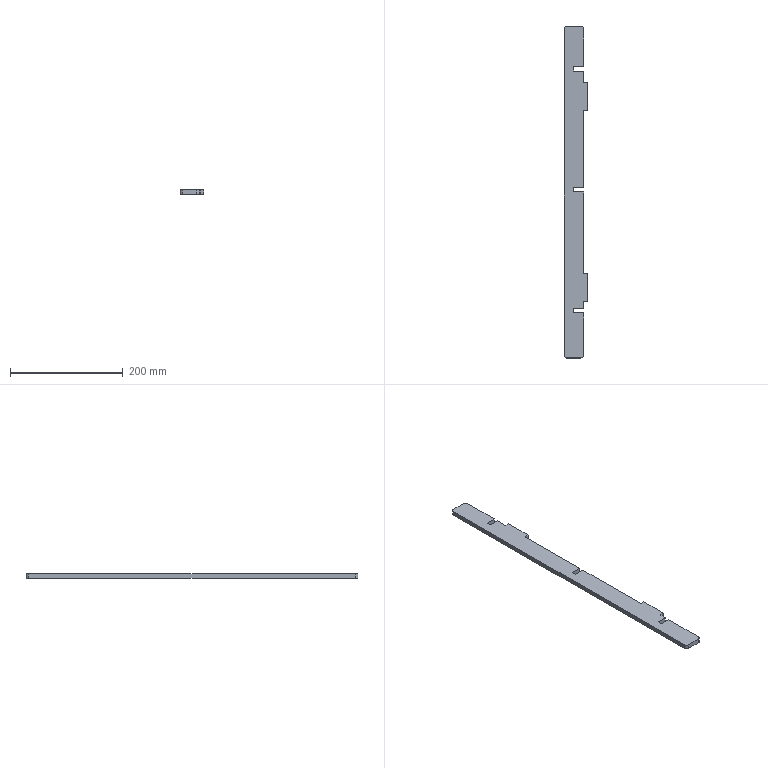Part | SolidWorks | features Fillet 2, FlatPattern 1, ICE 1, SMBaseFlange 1, SheetMetal 1 | 1 solid | 42 faces | box 42.5 x 590 x 8 mm | volume 167562 mm3 | plane 26 | cylinder 16 | commonest cylinder face diameters 2 x8 1 x4 10 x4
STEP:
#1=CARTESIAN_POINT('',(-612.5,244.764,0.));
#2=VERTEX_POINT('',#1);
#3=CARTESIAN_POINT('',(-612.5,263.685,0.));
#4=VERTEX_POINT('',#3);
#5=CARTESIAN_POINT('',(-612.5,243.685,0.));
#6=DIRECTION('',(0.,1.,0.));
#7=VECTOR('',#6,1000.);
#8=LINE('',#5,#7);
#9=EDGE_CURVE('',#2,#4,#8,.T.);
#10=ORIENTED_EDGE('',*,*,#9,.F.);
#11=CARTESIAN_POINT('',(-612.5,244.764,-8.));
#12=VERTEX_POINT('',#11);
#13=CARTESIAN_POINT('',(-612.5,244.764,-8.));
#14=DIRECTION('',(0.,0.,-1.));
#15=VECTOR('',#14,1000.);
#16=LINE('',#13,#15);
#17=EDGE_CURVE('',#2,#12,#16,.T.);
#18=ORIENTED_EDGE('',*,*,#17,.T.);
#19=CARTESIAN_POINT('',(-612.5,263.685,-8.));
#20=VERTEX_POINT('',#19);
#21=CARTESIAN_POINT('',(-612.5,243.685,-8.));
#22=DIRECTION('',(0.,1.,0.));
#23=VECTOR('',#22,1000.);
#24=LINE('',#21,#23);
#25=EDGE_CURVE('',#12,#20,#24,.T.);
#26=ORIENTED_EDGE('',*,*,#25,.T.);
#27=CARTESIAN_POINT('',(-612.5,263.685,-8.));
#28=DIRECTION('',(0.,0.,1.));
#29=VECTOR('',#28,1000.);
#30=LINE('',#27,#29);
#31=EDGE_CURVE('',#20,#4,#30,.T.);
#32=ORIENTED_EDGE('',*,*,#31,.T.);
#33=EDGE_LOOP('',(#10,#18,#26,#32));
#34=FACE_OUTER_BOUND('',#33,.T.);
#35=CARTESIAN_POINT('',(-612.5,243.685,-8.));
#36=DIRECTION('',(1.,0.,0.));
#37=DIRECTION('',(0.,1.,0.));
#38=AXIS2_PLACEMENT_3D('',#35,#36,#37);
#39=PLANE('',#38);
#40=ADVANCED_FACE('',(#34),#39,.T.);
#41=CARTESIAN_POINT('',(-605.,243.685,-8.));
#42=VERTEX_POINT('',#41);
#43=CARTESIAN_POINT('',(-611.421,243.685,-8.));
#44=VERTEX_POINT('',#43);
#45=CARTESIAN_POINT('',(-612.5,243.685,-8.));
#46=DIRECTION('',(-1.,0.,0.));
#47=VECTOR('',#46,1000.);
#48=LINE('',#45,#47);
#49=EDGE_CURVE('',#42,#44,#48,.T.);
#50=ORIENTED_EDGE('',*,*,#49,.T.);
#51=CARTESIAN_POINT('',(-611.421,243.685,0.));
#52=VERTEX_POINT('',#51);
#53=CARTESIAN_POINT('',(-611.421,243.685,-8.));
#54=DIRECTION('',(0.,0.,1.));
#55=VECTOR('',#54,1000.);
#56=LINE('',#53,#55);
#57=EDGE_CURVE('',#44,#52,#56,.T.);
#58=ORIENTED_EDGE('',*,*,#57,.T.);
#59=CARTESIAN_POINT('',(-605.,243.685,0.));
#60=VERTEX_POINT('',#59);
#61=CARTESIAN_POINT('',(-612.5,243.685,0.));
#62=DIRECTION('',(-1.,0.,0.));
#63=VECTOR('',#62,1000.);
#64=LINE('',#61,#63);
#65=EDGE_CURVE('',#60,#52,#64,.T.);
#66=ORIENTED_EDGE('',*,*,#65,.F.);
#67=CARTESIAN_POINT('',(-605.,243.685,-8.));
#68=DIRECTION('',(0.,0.,1.));
#69=VECTOR('',#68,1000.);
#70=LINE('',#67,#69);
#71=EDGE_CURVE('',#42,#60,#70,.T.);
#72=ORIENTED_EDGE('',*,*,#71,.F.);
#73=EDGE_LOOP('',(#50,#58,#66,#72));
#74=FACE_OUTER_BOUND('',#73,.T.);
#75=CARTESIAN_POINT('',(-612.5,243.685,-8.));
#76=DIRECTION('',(0.,1.,0.));
#77=DIRECTION('',(0.,0.,1.));
#78=AXIS2_PLACEMENT_3D('',#75,#76,#77);
#79=PLANE('',#78);
#80=ADVANCED_FACE('',(#74),#79,.T.);
#81=CARTESIAN_POINT('',(-611.421,193.685,0.));
#82=VERTEX_POINT('',#81);
#83=CARTESIAN_POINT('',(-605.,193.685,0.));
#84=VERTEX_POINT('',#83);
#85=CARTESIAN_POINT('',(-605.,193.685,0.));
#86=DIRECTION('',(1.,0.,0.));
#87=VECTOR('',#86,1000.);
#88=LINE('',#85,#87);
#89=EDGE_CURVE('',#82,#84,#88,.T.);
#90=ORIENTED_EDGE('',*,*,#89,.F.);
#91=CARTESIAN_POINT('',(-611.421,193.685,-8.));
#92=VERTEX_POINT('',#91);
#93=CARTESIAN_POINT('',(-611.421,193.685,-8.));
#94=DIRECTION('',(0.,0.,-1.));
#95=VECTOR('',#94,1000.);
#96=LINE('',#93,#95);
#97=EDGE_CURVE('',#82,#92,#96,.T.);
#98=ORIENTED_EDGE('',*,*,#97,.T.);
#99=CARTESIAN_POINT('',(-605.,193.685,-8.));
#100=VERTEX_POINT('',#99);
#101=CARTESIAN_POINT('',(-605.,193.685,-8.));
#102=DIRECTION('',(1.,0.,0.));
#103=VECTOR('',#102,1000.);
#104=LINE('',#101,#103);
#105=EDGE_CURVE('',#92,#100,#104,.T.);
#106=ORIENTED_EDGE('',*,*,#105,.T.);
#107=CARTESIAN_POINT('',(-605.,193.685,-8.));
#108=DIRECTION('',(0.,0.,1.));
#109=VECTOR('',#108,1000.);
#110=LINE('',#107,#109);
#111=EDGE_CURVE('',#100,#84,#110,.T.);
#112=ORIENTED_EDGE('',*,*,#111,.T.);
#113=EDGE_LOOP('',(#90,#98,#106,#112));
#114=FACE_OUTER_BOUND('',#113,.T.);
#115=CARTESIAN_POINT('',(-605.,193.685,-8.));
#116=DIRECTION('',(0.,-1.,0.));
#117=DIRECTION('',(0.,0.,-1.));
#118=AXIS2_PLACEMENT_3D('',#115,#116,#117);
#119=PLANE('',#118);
#120=ADVANCED_FACE('',(#114),#119,.T.);
#121=CARTESIAN_POINT('',(-612.5,56.685,-8.));
#122=VERTEX_POINT('',#121);
#123=CARTESIAN_POINT('',(-612.5,192.605,-8.));
#124=VERTEX_POINT('',#123);
#125=CARTESIAN_POINT('',(-612.5,56.685,-8.));
#126=DIRECTION('',(0.,1.,0.));
#127=VECTOR('',#126,1000.);
#128=LINE('',#125,#127);
#129=EDGE_CURVE('',#122,#124,#128,.T.);
#130=ORIENTED_EDGE('',*,*,#129,.T.);
#131=CARTESIAN_POINT('',(-612.5,192.605,0.));
#132=VERTEX_POINT('',#131);
#133=CARTESIAN_POINT('',(-612.5,192.605,-8.));
#134=DIRECTION('',(0.,0.,1.));
#135=VECTOR('',#134,1000.);
#136=LINE('',#133,#135);
#137=EDGE_CURVE('',#124,#132,#136,.T.);
#138=ORIENTED_EDGE('',*,*,#137,.T.);
#139=CARTESIAN_POINT('',(-612.5,56.685,0.));
#140=VERTEX_POINT('',#139);
#141=CARTESIAN_POINT('',(-612.5,56.685,0.));
#142=DIRECTION('',(0.,1.,0.));
#143=VECTOR('',#142,1000.);
#144=LINE('',#141,#143);
#145=EDGE_CURVE('',#140,#132,#144,.T.);
#146=ORIENTED_EDGE('',*,*,#145,.F.);
#147=CARTESIAN_POINT('',(-612.5,56.685,-8.));
#148=DIRECTION('',(0.,0.,1.));
#149=VECTOR('',#148,1000.);
#150=LINE('',#147,#149);
#151=EDGE_CURVE('',#122,#140,#150,.T.);
#152=ORIENTED_EDGE('',*,*,#151,.F.);
#153=EDGE_LOOP('',(#130,#138,#146,#152));
#154=FACE_OUTER_BOUND('',#153,.T.);
#155=CARTESIAN_POINT('',(-612.5,56.685,-8.));
#156=DIRECTION('',(1.,0.,0.));
#157=DIRECTION('',(0.,1.,0.));
#158=AXIS2_PLACEMENT_3D('',#155,#156,#157);
#159=PLANE('',#158);
#160=ADVANCED_FACE('',(#154),#159,.T.);
#161=CARTESIAN_POINT('',(-612.5,-95.236,0.));
#162=VERTEX_POINT('',#161);
#163=CARTESIAN_POINT('',(-612.5,48.685,0.));
#164=VERTEX_POINT('',#163);
#165=CARTESIAN_POINT('',(-612.5,-96.315,0.));
#166=DIRECTION('',(0.,1.,0.));
#167=VECTOR('',#166,1000.);
#168=LINE('',#165,#167);
#169=EDGE_CURVE('',#162,#164,#168,.T.);
#170=ORIENTED_EDGE('',*,*,#169,.F.);
#171=CARTESIAN_POINT('',(-612.5,-95.236,-8.));
#172=VERTEX_POINT('',#171);
#173=CARTESIAN_POINT('',(-612.5,-95.236,-8.));
#174=DIRECTION('',(0.,0.,-1.));
#175=VECTOR('',#174,1000.);
#176=LINE('',#173,#175);
#177=EDGE_CURVE('',#162,#172,#176,.T.);
#178=ORIENTED_EDGE('',*,*,#177,.T.);
#179=CARTESIAN_POINT('',(-612.5,48.685,-8.));
#180=VERTEX_POINT('',#179);
#181=CARTESIAN_POINT('',(-612.5,-96.315,-8.));
#182=DIRECTION('',(0.,1.,0.));
#183=VECTOR('',#182,1000.);
#184=LINE('',#181,#183);
#185=EDGE_CURVE('',#172,#180,#184,.T.);
#186=ORIENTED_EDGE('',*,*,#185,.T.);
#187=CARTESIAN_POINT('',(-612.5,48.685,-8.));
#188=DIRECTION('',(0.,0.,1.));
#189=VECTOR('',#188,1000.);
#190=LINE('',#187,#189);
#191=EDGE_CURVE('',#180,#164,#190,.T.);
#192=ORIENTED_EDGE('',*,*,#191,.T.);
#193=EDGE_LOOP('',(#170,#178,#186,#192));
#194=FACE_OUTER_BOUND('',#193,.T.);
#195=CARTESIAN_POINT('',(-612.5,-96.315,-8.));
#196=DIRECTION('',(1.,0.,0.));
#197=DIRECTION('',(0.,1.,0.));
#198=AXIS2_PLACEMENT_3D('',#195,#196,#197);
#199=PLANE('',#198);
#200=ADVANCED_FACE('',(#194),#199,.T.);
#201=CARTESIAN_POINT('',(-605.,-96.315,-8.));
#202=VERTEX_POINT('',#201);
#203=CARTESIAN_POINT('',(-611.421,-96.315,-8.));
#204=VERTEX_POINT('',#203);
#205=CARTESIAN_POINT('',(-612.5,-96.315,-8.));
#206=DIRECTION('',(-1.,0.,0.));
#207=VECTOR('',#206,1000.);
#208=LINE('',#205,#207);
#209=EDGE_CURVE('',#202,#204,#208,.T.);
#210=ORIENTED_EDGE('',*,*,#209,.T.);
#211=CARTESIAN_POINT('',(-611.421,-96.315,0.));
#212=VERTEX_POINT('',#211);
#213=CARTESIAN_POINT('',(-611.421,-96.315,-8.));
#214=DIRECTION('',(0.,0.,1.));
#215=VECTOR('',#214,1000.);
#216=LINE('',#213,#215);
#217=EDGE_CURVE('',#204,#212,#216,.T.);
#218=ORIENTED_EDGE('',*,*,#217,.T.);
#219=CARTESIAN_POINT('',(-605.,-96.315,0.));
#220=VERTEX_POINT('',#219);
#221=CARTESIAN_POINT('',(-612.5,-96.315,0.));
#222=DIRECTION('',(-1.,0.,0.));
#223=VECTOR('',#222,1000.);
#224=LINE('',#221,#223);
#225=EDGE_CURVE('',#220,#212,#224,.T.);
#226=ORIENTED_EDGE('',*,*,#225,.F.);
#227=CARTESIAN_POINT('',(-605.,-96.315,-8.));
#228=DIRECTION('',(0.,0.,1.));
#229=VECTOR('',#228,1000.);
#230=LINE('',#227,#229);
#231=EDGE_CURVE('',#202,#220,#230,.T.);
#232=ORIENTED_EDGE('',*,*,#231,.F.);
#233=EDGE_LOOP('',(#210,#218,#226,#232));
#234=FACE_OUTER_BOUND('',#233,.T.);
#235=CARTESIAN_POINT('',(-612.5,-96.315,-8.));
#236=DIRECTION('',(0.,1.,0.));
#237=DIRECTION('',(0.,0.,1.));
#238=AXIS2_PLACEMENT_3D('',#235,#236,#237);
#239=PLANE('',#238);
#240=ADVANCED_FACE('',(#234),#239,.T.);
#241=CARTESIAN_POINT('',(-611.421,-146.315,0.));
#242=VERTEX_POINT('',#241);
#243=CARTESIAN_POINT('',(-605.,-146.315,0.));
#244=VERTEX_POINT('',#243);
#245=CARTESIAN_POINT('',(-605.,-146.315,0.));
#246=DIRECTION('',(1.,0.,0.));
#247=VECTOR('',#246,1000.);
#248=LINE('',#245,#247);
#249=EDGE_CURVE('',#242,#244,#248,.T.);
#250=ORIENTED_EDGE('',*,*,#249,.F.);
#251=CARTESIAN_POINT('',(-611.421,-146.315,-8.));
#252=VERTEX_POINT('',#251);
#253=CARTESIAN_POINT('',(-611.421,-146.315,-8.));
#254=DIRECTION('',(0.,0.,-1.));
#255=VECTOR('',#254,1000.);
#256=LINE('',#253,#255);
#257=EDGE_CURVE('',#242,#252,#256,.T.);
#258=ORIENTED_EDGE('',*,*,#257,.T.);
#259=CARTESIAN_POINT('',(-605.,-146.315,-8.));
#260=VERTEX_POINT('',#259);
#261=CARTESIAN_POINT('',(-605.,-146.315,-8.));
#262=DIRECTION('',(1.,0.,0.));
#263=VECTOR('',#262,1000.);
#264=LINE('',#261,#263);
#265=EDGE_CURVE('',#252,#260,#264,.T.);
#266=ORIENTED_EDGE('',*,*,#265,.T.);
#267=CARTESIAN_POINT('',(-605.,-146.315,-8.));
#268=DIRECTION('',(0.,0.,1.));
#269=VECTOR('',#268,1000.);
#270=LINE('',#267,#269);
#271=EDGE_CURVE('',#260,#244,#270,.T.);
#272=ORIENTED_EDGE('',*,*,#271,.T.);
#273=EDGE_LOOP('',(#250,#258,#266,#272));
#274=FACE_OUTER_BOUND('',#273,.T.);
#275=CARTESIAN_POINT('',(-605.,-146.315,-8.));
#276=DIRECTION('',(0.,-1.,0.));
#277=DIRECTION('',(0.,0.,-1.));
#278=AXIS2_PLACEMENT_3D('',#275,#276,#277);
#279=PLANE('',#278);
#280=ADVANCED_FACE('',(#274),#279,.T.);
#281=CARTESIAN_POINT('',(-612.5,-158.315,-8.));
#282=VERTEX_POINT('',#281);
#283=CARTESIAN_POINT('',(-612.5,-147.395,-8.));
#284=VERTEX_POINT('',#283);
#285=CARTESIAN_POINT('',(-612.5,-158.315,-8.));
#286=DIRECTION('',(0.,1.,0.));
#287=VECTOR('',#286,1000.);
#288=LINE('',#285,#287);
#289=EDGE_CURVE('',#282,#284,#288,.T.);
#290=ORIENTED_EDGE('',*,*,#289,.T.);
#291=CARTESIAN_POINT('',(-612.5,-147.395,0.));
#292=VERTEX_POINT('',#291);
#293=CARTESIAN_POINT('',(-612.5,-147.395,-8.));
#294=DIRECTION('',(0.,0.,1.));
#295=VECTOR('',#294,1000.);
#296=LINE('',#293,#295);
#297=EDGE_CURVE('',#284,#292,#296,.T.);
#298=ORIENTED_EDGE('',*,*,#297,.T.);
#299=CARTESIAN_POINT('',(-612.5,-158.315,0.));
#300=VERTEX_POINT('',#299);
#301=CARTESIAN_POINT('',(-612.5,-158.315,0.));
#302=DIRECTION('',(0.,1.,0.));
#303=VECTOR('',#302,1000.);
#304=LINE('',#301,#303);
#305=EDGE_CURVE('',#300,#292,#304,.T.);
#306=ORIENTED_EDGE('',*,*,#305,.F.);
#307=CARTESIAN_POINT('',(-612.5,-158.315,-8.));
#308=DIRECTION('',(0.,0.,1.));
#309=VECTOR('',#308,1000.);
#310=LINE('',#307,#309);
#311=EDGE_CURVE('',#282,#300,#310,.T.);
#312=ORIENTED_EDGE('',*,*,#311,.F.);
#313=EDGE_LOOP('',(#290,#298,#306,#312));
#314=FACE_OUTER_BOUND('',#313,.T.);
#315=CARTESIAN_POINT('',(-612.5,-158.315,-8.));
#316=DIRECTION('',(1.,0.,0.));
#317=DIRECTION('',(0.,1.,0.));
#318=AXIS2_PLACEMENT_3D('',#315,#316,#317);
#319=PLANE('',#318);
#320=ADVANCED_FACE('',(#314),#319,.T.);
#321=ORIENTED_EDGE('',*,*,#105,.F.);
#322=CARTESIAN_POINT('',(-611.974,193.851,-8.));
#323=VERTEX_POINT('',#322);
#324=CARTESIAN_POINT('',(-611.421,194.685,-8.));
#325=DIRECTION('',(0.,0.,-1.));
#326=DIRECTION('',(1.,0.,0.));
#327=AXIS2_PLACEMENT_3D('',#324,#325,#326);
#328=CIRCLE('',#327,1.);
#329=EDGE_CURVE('',#92,#323,#328,.T.);
#330=ORIENTED_EDGE('',*,*,#329,.T.);
#331=CARTESIAN_POINT('',(-612.667,193.158,-8.));
#332=VERTEX_POINT('',#331);
#333=CARTESIAN_POINT('',(-612.25,193.435,-8.));
#334=DIRECTION('',(0.,0.,1.));
#335=DIRECTION('',(1.,0.,0.));
#336=AXIS2_PLACEMENT_3D('',#333,#334,#335);
#337=CIRCLE('',#336,0.5);
#338=EDGE_CURVE('',#323,#332,#337,.T.);
#339=ORIENTED_EDGE('',*,*,#338,.T.);
#340=CARTESIAN_POINT('',(-613.5,192.605,-8.));
#341=DIRECTION('',(0.,0.,-1.));
#342=DIRECTION('',(1.,0.,0.));
#343=AXIS2_PLACEMENT_3D('',#340,#341,#342);
#344=CIRCLE('',#343,1.);
#345=EDGE_CURVE('',#332,#124,#344,.T.);
#346=ORIENTED_EDGE('',*,*,#345,.T.);
#347=ORIENTED_EDGE('',*,*,#129,.F.);
#348=CARTESIAN_POINT('',(-630.5,56.685,-8.));
#349=VERTEX_POINT('',#348);
#350=CARTESIAN_POINT('',(-630.5,56.685,-8.));
#351=DIRECTION('',(1.,0.,0.));
#352=VECTOR('',#351,1000.);
#353=LINE('',#350,#352);
#354=EDGE_CURVE('',#349,#122,#353,.T.);
#355=ORIENTED_EDGE('',*,*,#354,.F.);
#356=CARTESIAN_POINT('',(-630.5,48.685,-8.));
#357=VERTEX_POINT('',#356);
#358=CARTESIAN_POINT('',(-630.5,48.685,-8.));
#359=DIRECTION('',(0.,1.,0.));
#360=VECTOR('',#359,1000.);
#361=LINE('',#358,#360);
#362=EDGE_CURVE('',#357,#349,#361,.T.);
#363=ORIENTED_EDGE('',*,*,#362,.F.);
#364=CARTESIAN_POINT('',(-612.5,48.685,-8.));
#365=DIRECTION('',(-1.,0.,0.));
#366=VECTOR('',#365,1000.);
#367=LINE('',#364,#366);
#368=EDGE_CURVE('',#180,#357,#367,.T.);
#369=ORIENTED_EDGE('',*,*,#368,.F.);
#370=ORIENTED_EDGE('',*,*,#185,.F.);
#371=CARTESIAN_POINT('',(-612.667,-95.789,-8.));
#372=VERTEX_POINT('',#371);
#373=CARTESIAN_POINT('',(-613.5,-95.236,-8.));
#374=DIRECTION('',(0.,0.,-1.));
#375=DIRECTION('',(1.,0.,0.));
#376=AXIS2_PLACEMENT_3D('',#373,#374,#375);
#377=CIRCLE('',#376,1.);
#378=EDGE_CURVE('',#172,#372,#377,.T.);
#379=ORIENTED_EDGE('',*,*,#378,.T.);
#380=CARTESIAN_POINT('',(-611.974,-96.482,-8.));
#381=VERTEX_POINT('',#380);
#382=CARTESIAN_POINT('',(-612.25,-96.065,-8.));
#383=DIRECTION('',(0.,0.,1.));
#384=DIRECTION('',(1.,0.,0.));
#385=AXIS2_PLACEMENT_3D('',#382,#383,#384);
#386=CIRCLE('',#385,0.5);
#387=EDGE_CURVE('',#372,#381,#386,.T.);
#388=ORIENTED_EDGE('',*,*,#387,.T.);
#389=CARTESIAN_POINT('',(-611.421,-97.315,-8.));
#390=DIRECTION('',(0.,0.,-1.));
#391=DIRECTION('',(1.,0.,0.));
#392=AXIS2_PLACEMENT_3D('',#389,#390,#391);
#393=CIRCLE('',#392,1.);
#394=EDGE_CURVE('',#381,#204,#393,.T.);
#395=ORIENTED_EDGE('',*,*,#394,.T.);
#396=ORIENTED_EDGE('',*,*,#209,.F.);
#397=CARTESIAN_POINT('',(-605.,-96.315,-8.));
#398=DIRECTION('',(0.,1.,0.));
#399=VECTOR('',#398,1000.);
#400=LINE('',#397,#399);
#401=EDGE_CURVE('',#260,#202,#400,.T.);
#402=ORIENTED_EDGE('',*,*,#401,.F.);
#403=ORIENTED_EDGE('',*,*,#265,.F.);
#404=CARTESIAN_POINT('',(-611.974,-146.149,-8.));
#405=VERTEX_POINT('',#404);
#406=CARTESIAN_POINT('',(-611.421,-145.315,-8.));
#407=DIRECTION('',(0.,0.,-1.));
#408=DIRECTION('',(1.,0.,0.));
#409=AXIS2_PLACEMENT_3D('',#406,#407,#408);
#410=CIRCLE('',#409,1.);
#411=EDGE_CURVE('',#252,#405,#410,.T.);
#412=ORIENTED_EDGE('',*,*,#411,.T.);
#413=CARTESIAN_POINT('',(-612.667,-146.842,-8.));
#414=VERTEX_POINT('',#413);
#415=CARTESIAN_POINT('',(-612.25,-146.565,-8.));
#416=DIRECTION('',(0.,0.,1.));
#417=DIRECTION('',(1.,0.,0.));
#418=AXIS2_PLACEMENT_3D('',#415,#416,#417);
#419=CIRCLE('',#418,0.5);
#420=EDGE_CURVE('',#405,#414,#419,.T.);
#421=ORIENTED_EDGE('',*,*,#420,.T.);
#422=CARTESIAN_POINT('',(-613.5,-147.395,-8.));
#423=DIRECTION('',(0.,0.,-1.));
#424=DIRECTION('',(1.,0.,0.));
#425=AXIS2_PLACEMENT_3D('',#422,#423,#424);
#426=CIRCLE('',#425,1.);
#427=EDGE_CURVE('',#414,#284,#426,.T.);
#428=ORIENTED_EDGE('',*,*,#427,.T.);
#429=ORIENTED_EDGE('',*,*,#289,.F.);
#430=CARTESIAN_POINT('',(-630.5,-158.315,-8.));
#431=VERTEX_POINT('',#430);
#432=CARTESIAN_POINT('',(-612.5,-158.315,-8.));
#433=DIRECTION('',(1.,0.,0.));
#434=VECTOR('',#433,1000.);
#435=LINE('',#432,#434);
#436=EDGE_CURVE('',#431,#282,#435,.T.);
#437=ORIENTED_EDGE('',*,*,#436,.F.);
#438=CARTESIAN_POINT('',(-630.5,-166.315,-8.));
#439=VERTEX_POINT('',#438);
#440=CARTESIAN_POINT('',(-630.5,-158.315,-8.));
#441=DIRECTION('',(0.,1.,0.));
#442=VECTOR('',#441,1000.);
#443=LINE('',#440,#442);
#444=EDGE_CURVE('',#439,#431,#443,.T.);
#445=ORIENTED_EDGE('',*,*,#444,.F.);
#446=CARTESIAN_POINT('',(-612.5,-166.315,-8.));
#447=VERTEX_POINT('',#446);
#448=CARTESIAN_POINT('',(-630.5,-166.315,-8.));
#449=DIRECTION('',(-1.,0.,0.));
#450=VECTOR('',#449,1000.);
#451=LINE('',#448,#450);
#452=EDGE_CURVE('',#447,#439,#451,.T.);
#453=ORIENTED_EDGE('',*,*,#452,.F.);
#454=CARTESIAN_POINT('',(-612.5,-241.315,-8.));
#455=VERTEX_POINT('',#454);
#456=CARTESIAN_POINT('',(-612.5,-246.315,-8.));
#457=DIRECTION('',(0.,1.,0.));
#458=VECTOR('',#457,1000.);
#459=LINE('',#456,#458);
#460=EDGE_CURVE('',#455,#447,#459,.T.);
#461=ORIENTED_EDGE('',*,*,#460,.F.);
#462=CARTESIAN_POINT('',(-617.5,-246.315,-8.));
#463=VERTEX_POINT('',#462);
#464=CARTESIAN_POINT('',(-617.5,-241.315,-8.));
#465=DIRECTION('',(0.,0.,-1.));
#466=DIRECTION('',(1.,0.,0.));
#467=AXIS2_PLACEMENT_3D('',#464,#465,#466);
#468=CIRCLE('',#467,5.);
#469=EDGE_CURVE('',#455,#463,#468,.T.);
#470=ORIENTED_EDGE('',*,*,#469,.T.);
#471=CARTESIAN_POINT('',(-642.5,-246.315,-8.));
#472=VERTEX_POINT('',#471);
#473=CARTESIAN_POINT('',(-647.5,-246.315,-8.));
#474=DIRECTION('',(1.,0.,0.));
#475=VECTOR('',#474,1000.);
#476=LINE('',#473,#475);
#477=EDGE_CURVE('',#472,#463,#476,.T.);
#478=ORIENTED_EDGE('',*,*,#477,.F.);
#479=CARTESIAN_POINT('',(-647.5,-241.315,-8.));
#480=VERTEX_POINT('',#479);
#481=CARTESIAN_POINT('',(-642.5,-241.315,-8.));
#482=DIRECTION('',(0.,0.,-1.));
#483=DIRECTION('',(1.,0.,0.));
#484=AXIS2_PLACEMENT_3D('',#481,#482,#483);
#485=CIRCLE('',#484,5.);
#486=EDGE_CURVE('',#472,#480,#485,.T.);
#487=ORIENTED_EDGE('',*,*,#486,.T.);
#488=CARTESIAN_POINT('',(-647.5,338.685,-8.));
#489=VERTEX_POINT('',#488);
#490=CARTESIAN_POINT('',(-647.5,343.685,-8.));
#491=DIRECTION('',(0.,-1.,0.));
#492=VECTOR('',#491,1000.);
#493=LINE('',#490,#492);
#494=EDGE_CURVE('',#489,#480,#493,.T.);
#495=ORIENTED_EDGE('',*,*,#494,.F.);
#496=CARTESIAN_POINT('',(-642.5,343.685,-8.));
#497=VERTEX_POINT('',#496);
#498=CARTESIAN_POINT('',(-642.5,338.685,-8.));
#499=DIRECTION('',(0.,0.,-1.));
#500=DIRECTION('',(1.,0.,0.));
#501=AXIS2_PLACEMENT_3D('',#498,#499,#500);
#502=CIRCLE('',#501,5.);
#503=EDGE_CURVE('',#489,#497,#502,.T.);
#504=ORIENTED_EDGE('',*,*,#503,.T.);
#505=CARTESIAN_POINT('',(-617.5,343.685,-8.));
#506=VERTEX_POINT('',#505);
#507=CARTESIAN_POINT('',(-612.5,343.685,-8.));
#508=DIRECTION('',(-1.,0.,0.));
#509=VECTOR('',#508,1000.);
#510=LINE('',#507,#509);
#511=EDGE_CURVE('',#506,#497,#510,.T.);
#512=ORIENTED_EDGE('',*,*,#511,.F.);
#513=CARTESIAN_POINT('',(-612.5,338.685,-8.));
#514=VERTEX_POINT('',#513);
#515=CARTESIAN_POINT('',(-617.5,338.685,-8.));
#516=DIRECTION('',(0.,0.,-1.));
#517=DIRECTION('',(1.,0.,0.));
#518=AXIS2_PLACEMENT_3D('',#515,#516,#517);
#519=CIRCLE('',#518,5.);
#520=EDGE_CURVE('',#506,#514,#519,.T.);
#521=ORIENTED_EDGE('',*,*,#520,.T.);
#522=CARTESIAN_POINT('',(-612.5,271.685,-8.));
#523=VERTEX_POINT('',#522);
#524=CARTESIAN_POINT('',(-612.5,271.685,-8.));
#525=DIRECTION('',(0.,1.,0.));
#526=VECTOR('',#525,1000.);
#527=LINE('',#524,#526);
#528=EDGE_CURVE('',#523,#514,#527,.T.);
#529=ORIENTED_EDGE('',*,*,#528,.F.);
#530=CARTESIAN_POINT('',(-630.5,271.685,-8.));
#531=VERTEX_POINT('',#530);
#532=CARTESIAN_POINT('',(-630.5,271.685,-8.));
#533=DIRECTION('',(1.,0.,0.));
#534=VECTOR('',#533,1000.);
#535=LINE('',#532,#534);
#536=EDGE_CURVE('',#531,#523,#535,.T.);
#537=ORIENTED_EDGE('',*,*,#536,.F.);
#538=CARTESIAN_POINT('',(-630.5,263.685,-8.));
#539=VERTEX_POINT('',#538);
#540=CARTESIAN_POINT('',(-630.5,263.685,-8.));
#541=DIRECTION('',(0.,1.,0.));
#542=VECTOR('',#541,1000.);
#543=LINE('',#540,#542);
#544=EDGE_CURVE('',#539,#531,#543,.T.);
#545=ORIENTED_EDGE('',*,*,#544,.F.);
#546=CARTESIAN_POINT('',(-612.5,263.685,-8.));
#547=DIRECTION('',(-1.,0.,0.));
#548=VECTOR('',#547,1000.);
#549=LINE('',#546,#548);
#550=EDGE_CURVE('',#20,#539,#549,.T.);
#551=ORIENTED_EDGE('',*,*,#550,.F.);
#552=ORIENTED_EDGE('',*,*,#25,.F.);
#553=CARTESIAN_POINT('',(-612.667,244.211,-8.));
#554=VERTEX_POINT('',#553);
#555=CARTESIAN_POINT('',(-613.5,244.764,-8.));
#556=DIRECTION('',(0.,0.,-1.));
#557=DIRECTION('',(1.,0.,0.));
#558=AXIS2_PLACEMENT_3D('',#555,#556,#557);
#559=CIRCLE('',#558,1.);
#560=EDGE_CURVE('',#12,#554,#559,.T.);
#561=ORIENTED_EDGE('',*,*,#560,.T.);
#562=CARTESIAN_POINT('',(-611.974,243.518,-8.));
#563=VERTEX_POINT('',#562);
#564=CARTESIAN_POINT('',(-612.25,243.935,-8.));
#565=DIRECTION('',(0.,0.,1.));
#566=DIRECTION('',(1.,0.,0.));
#567=AXIS2_PLACEMENT_3D('',#564,#565,#566);
#568=CIRCLE('',#567,0.5);
#569=EDGE_CURVE('',#554,#563,#568,.T.);
#570=ORIENTED_EDGE('',*,*,#569,.T.);
#571=CARTESIAN_POINT('',(-611.421,242.685,-8.));
#572=DIRECTION('',(0.,0.,-1.));
#573=DIRECTION('',(1.,0.,0.));
#574=AXIS2_PLACEMENT_3D('',#571,#572,#573);
#575=CIRCLE('',#574,1.);
#576=EDGE_CURVE('',#563,#44,#575,.T.);
#577=ORIENTED_EDGE('',*,*,#576,.T.);
#578=ORIENTED_EDGE('',*,*,#49,.F.);
#579=CARTESIAN_POINT('',(-605.,243.685,-8.));
#580=DIRECTION('',(0.,1.,0.));
#581=VECTOR('',#580,1000.);
#582=LINE('',#579,#581);
#583=EDGE_CURVE('',#100,#42,#582,.T.);
#584=ORIENTED_EDGE('',*,*,#583,.F.);
#585=EDGE_LOOP('',(#321,#330,#339,#346,#347,#355,#363,#369,#370,#379,#388,#395,#396,#402,#403,#412,#421,#428,#429,#437,#445,#453,#461,#470,#478,#487,#495,#504,#512,#521,#529,#537,#545,#551,#552,#561,#570,#577,#578,#584));
#586=FACE_OUTER_BOUND('',#585,.T.);
#587=CARTESIAN_POINT('',(0.,0.,-8.));
#588=DIRECTION('',(0.,0.,1.));
#589=DIRECTION('',(1.,0.,0.));
#590=AXIS2_PLACEMENT_3D('',#587,#588,#589);
#591=PLANE('',#590);
#592=ADVANCED_FACE('',(#586),#591,.F.);
#593=CARTESIAN_POINT('',(-611.974,193.851,0.));
#594=VERTEX_POINT('',#593);
#595=CARTESIAN_POINT('',(-612.667,193.158,0.));
#596=VERTEX_POINT('',#595);
#597=CARTESIAN_POINT('',(-612.25,193.435,0.));
#598=DIRECTION('',(0.,0.,1.));
#599=DIRECTION('',(1.,0.,0.));
#600=AXIS2_PLACEMENT_3D('',#597,#598,#599);
#601=CIRCLE('',#600,0.5);
#602=EDGE_CURVE('',#594,#596,#601,.T.);
#603=ORIENTED_EDGE('',*,*,#602,.F.);
#604=CARTESIAN_POINT('',(-611.421,194.685,0.));
#605=DIRECTION('',(0.,0.,1.));
#606=DIRECTION('',(1.,0.,0.));
#607=AXIS2_PLACEMENT_3D('',#604,#605,#606);
#608=CIRCLE('',#607,1.);
#609=EDGE_CURVE('',#594,#82,#608,.T.);
#610=ORIENTED_EDGE('',*,*,#609,.T.);
#611=ORIENTED_EDGE('',*,*,#89,.T.);
#612=CARTESIAN_POINT('',(-605.,243.685,0.));
#613=DIRECTION('',(0.,1.,0.));
#614=VECTOR('',#613,1000.);
#615=LINE('',#612,#614);
#616=EDGE_CURVE('',#84,#60,#615,.T.);
#617=ORIENTED_EDGE('',*,*,#616,.T.);
#618=ORIENTED_EDGE('',*,*,#65,.T.);
#619=CARTESIAN_POINT('',(-611.974,243.518,0.));
#620=VERTEX_POINT('',#619);
#621=CARTESIAN_POINT('',(-611.421,242.685,0.));
#622=DIRECTION('',(0.,0.,1.));
#623=DIRECTION('',(1.,0.,0.));
#624=AXIS2_PLACEMENT_3D('',#621,#622,#623);
#625=CIRCLE('',#624,1.);
#626=EDGE_CURVE('',#52,#620,#625,.T.);
#627=ORIENTED_EDGE('',*,*,#626,.T.);
#628=CARTESIAN_POINT('',(-612.667,244.211,0.));
#629=VERTEX_POINT('',#628);
#630=CARTESIAN_POINT('',(-612.25,243.935,0.));
#631=DIRECTION('',(0.,0.,1.));
#632=DIRECTION('',(1.,0.,0.));
#633=AXIS2_PLACEMENT_3D('',#630,#631,#632);
#634=CIRCLE('',#633,0.5);
#635=EDGE_CURVE('',#629,#620,#634,.T.);
#636=ORIENTED_EDGE('',*,*,#635,.F.);
#637=CARTESIAN_POINT('',(-613.5,244.764,0.));
#638=DIRECTION('',(0.,0.,1.));
#639=DIRECTION('',(1.,0.,0.));
#640=AXIS2_PLACEMENT_3D('',#637,#638,#639);
#641=CIRCLE('',#640,1.);
#642=EDGE_CURVE('',#629,#2,#641,.T.);
#643=ORIENTED_EDGE('',*,*,#642,.T.);
#644=ORIENTED_EDGE('',*,*,#9,.T.);
#645=CARTESIAN_POINT('',(-630.5,263.685,0.));
#646=VERTEX_POINT('',#645);
#647=CARTESIAN_POINT('',(-612.5,263.685,0.));
#648=DIRECTION('',(-1.,0.,0.));
#649=VECTOR('',#648,1000.);
#650=LINE('',#647,#649);
#651=EDGE_CURVE('',#4,#646,#650,.T.);
#652=ORIENTED_EDGE('',*,*,#651,.T.);
#653=CARTESIAN_POINT('',(-630.5,271.685,0.));
#654=VERTEX_POINT('',#653);
#655=CARTESIAN_POINT('',(-630.5,263.685,0.));
#656=DIRECTION('',(0.,1.,0.));
#657=VECTOR('',#656,1000.);
#658=LINE('',#655,#657);
#659=EDGE_CURVE('',#646,#654,#658,.T.);
#660=ORIENTED_EDGE('',*,*,#659,.T.);
#661=CARTESIAN_POINT('',(-612.5,271.685,0.));
#662=VERTEX_POINT('',#661);
#663=CARTESIAN_POINT('',(-630.5,271.685,0.));
#664=DIRECTION('',(1.,0.,0.));
#665=VECTOR('',#664,1000.);
#666=LINE('',#663,#665);
#667=EDGE_CURVE('',#654,#662,#666,.T.);
#668=ORIENTED_EDGE('',*,*,#667,.T.);
#669=CARTESIAN_POINT('',(-612.5,338.685,0.));
#670=VERTEX_POINT('',#669);
#671=CARTESIAN_POINT('',(-612.5,271.685,0.));
#672=DIRECTION('',(0.,1.,0.));
#673=VECTOR('',#672,1000.);
#674=LINE('',#671,#673);
#675=EDGE_CURVE('',#662,#670,#674,.T.);
#676=ORIENTED_EDGE('',*,*,#675,.T.);
#677=CARTESIAN_POINT('',(-617.5,343.685,0.));
#678=VERTEX_POINT('',#677);
#679=CARTESIAN_POINT('',(-617.5,338.685,0.));
#680=DIRECTION('',(0.,0.,1.));
#681=DIRECTION('',(1.,0.,0.));
#682=AXIS2_PLACEMENT_3D('',#679,#680,#681);
#683=CIRCLE('',#682,5.);
#684=EDGE_CURVE('',#670,#678,#683,.T.);
#685=ORIENTED_EDGE('',*,*,#684,.T.);
#686=CARTESIAN_POINT('',(-642.5,343.685,0.));
#687=VERTEX_POINT('',#686);
#688=CARTESIAN_POINT('',(-612.5,343.685,0.));
#689=DIRECTION('',(-1.,0.,0.));
#690=VECTOR('',#689,1000.);
#691=LINE('',#688,#690);
#692=EDGE_CURVE('',#678,#687,#691,.T.);
#693=ORIENTED_EDGE('',*,*,#692,.T.);
#694=CARTESIAN_POINT('',(-647.5,338.685,0.));
#695=VERTEX_POINT('',#694);
#696=CARTESIAN_POINT('',(-642.5,338.685,0.));
#697=DIRECTION('',(0.,0.,1.));
#698=DIRECTION('',(1.,0.,0.));
#699=AXIS2_PLACEMENT_3D('',#696,#697,#698);
#700=CIRCLE('',#699,5.);
#701=EDGE_CURVE('',#687,#695,#700,.T.);
#702=ORIENTED_EDGE('',*,*,#701,.T.);
#703=CARTESIAN_POINT('',(-647.5,-241.315,0.));
#704=VERTEX_POINT('',#703);
#705=CARTESIAN_POINT('',(-647.5,343.685,0.));
#706=DIRECTION('',(0.,-1.,0.));
#707=VECTOR('',#706,1000.);
#708=LINE('',#705,#707);
#709=EDGE_CURVE('',#695,#704,#708,.T.);
#710=ORIENTED_EDGE('',*,*,#709,.T.);
#711=CARTESIAN_POINT('',(-642.5,-246.315,0.));
#712=VERTEX_POINT('',#711);
#713=CARTESIAN_POINT('',(-642.5,-241.315,0.));
#714=DIRECTION('',(0.,0.,1.));
#715=DIRECTION('',(1.,0.,0.));
#716=AXIS2_PLACEMENT_3D('',#713,#714,#715);
#717=CIRCLE('',#716,5.);
#718=EDGE_CURVE('',#704,#712,#717,.T.);
#719=ORIENTED_EDGE('',*,*,#718,.T.);
#720=CARTESIAN_POINT('',(-617.5,-246.315,0.));
#721=VERTEX_POINT('',#720);
#722=CARTESIAN_POINT('',(-647.5,-246.315,0.));
#723=DIRECTION('',(1.,0.,0.));
#724=VECTOR('',#723,1000.);
#725=LINE('',#722,#724);
#726=EDGE_CURVE('',#712,#721,#725,.T.);
#727=ORIENTED_EDGE('',*,*,#726,.T.);
#728=CARTESIAN_POINT('',(-612.5,-241.315,0.));
#729=VERTEX_POINT('',#728);
#730=CARTESIAN_POINT('',(-617.5,-241.315,0.));
#731=DIRECTION('',(0.,0.,1.));
#732=DIRECTION('',(1.,0.,0.));
#733=AXIS2_PLACEMENT_3D('',#730,#731,#732);
#734=CIRCLE('',#733,5.);
#735=EDGE_CURVE('',#721,#729,#734,.T.);
#736=ORIENTED_EDGE('',*,*,#735,.T.);
#737=CARTESIAN_POINT('',(-612.5,-166.315,0.));
#738=VERTEX_POINT('',#737);
#739=CARTESIAN_POINT('',(-612.5,-246.315,0.));
#740=DIRECTION('',(0.,1.,0.));
#741=VECTOR('',#740,1000.);
#742=LINE('',#739,#741);
#743=EDGE_CURVE('',#729,#738,#742,.T.);
#744=ORIENTED_EDGE('',*,*,#743,.T.);
#745=CARTESIAN_POINT('',(-630.5,-166.315,0.));
#746=VERTEX_POINT('',#745);
#747=CARTESIAN_POINT('',(-630.5,-166.315,0.));
#748=DIRECTION('',(-1.,0.,0.));
#749=VECTOR('',#748,1000.);
#750=LINE('',#747,#749);
#751=EDGE_CURVE('',#738,#746,#750,.T.);
#752=ORIENTED_EDGE('',*,*,#751,.T.);
#753=CARTESIAN_POINT('',(-630.5,-158.315,0.));
#754=VERTEX_POINT('',#753);
#755=CARTESIAN_POINT('',(-630.5,-158.315,0.));
#756=DIRECTION('',(0.,1.,0.));
#757=VECTOR('',#756,1000.);
#758=LINE('',#755,#757);
#759=EDGE_CURVE('',#746,#754,#758,.T.);
#760=ORIENTED_EDGE('',*,*,#759,.T.);
#761=CARTESIAN_POINT('',(-612.5,-158.315,0.));
#762=DIRECTION('',(1.,0.,0.));
#763=VECTOR('',#762,1000.);
#764=LINE('',#761,#763);
#765=EDGE_CURVE('',#754,#300,#764,.T.);
#766=ORIENTED_EDGE('',*,*,#765,.T.);
#767=ORIENTED_EDGE('',*,*,#305,.T.);
#768=CARTESIAN_POINT('',(-612.667,-146.842,0.));
#769=VERTEX_POINT('',#768);
#770=CARTESIAN_POINT('',(-613.5,-147.395,0.));
#771=DIRECTION('',(0.,0.,1.));
#772=DIRECTION('',(1.,0.,0.));
#773=AXIS2_PLACEMENT_3D('',#770,#771,#772);
#774=CIRCLE('',#773,1.);
#775=EDGE_CURVE('',#292,#769,#774,.T.);
#776=ORIENTED_EDGE('',*,*,#775,.T.);
#777=CARTESIAN_POINT('',(-611.974,-146.149,0.));
#778=VERTEX_POINT('',#777);
#779=CARTESIAN_POINT('',(-612.25,-146.565,0.));
#780=DIRECTION('',(0.,0.,1.));
#781=DIRECTION('',(1.,0.,0.));
#782=AXIS2_PLACEMENT_3D('',#779,#780,#781);
#783=CIRCLE('',#782,0.5);
#784=EDGE_CURVE('',#778,#769,#783,.T.);
#785=ORIENTED_EDGE('',*,*,#784,.F.);
#786=CARTESIAN_POINT('',(-611.421,-145.315,0.));
#787=DIRECTION('',(0.,0.,1.));
#788=DIRECTION('',(1.,0.,0.));
#789=AXIS2_PLACEMENT_3D('',#786,#787,#788);
#790=CIRCLE('',#789,1.);
#791=EDGE_CURVE('',#778,#242,#790,.T.);
#792=ORIENTED_EDGE('',*,*,#791,.T.);
#793=ORIENTED_EDGE('',*,*,#249,.T.);
#794=CARTESIAN_POINT('',(-605.,-96.315,0.));
#795=DIRECTION('',(0.,1.,0.));
#796=VECTOR('',#795,1000.);
#797=LINE('',#794,#796);
#798=EDGE_CURVE('',#244,#220,#797,.T.);
#799=ORIENTED_EDGE('',*,*,#798,.T.);
#800=ORIENTED_EDGE('',*,*,#225,.T.);
#801=CARTESIAN_POINT('',(-611.974,-96.482,0.));
#802=VERTEX_POINT('',#801);
#803=CARTESIAN_POINT('',(-611.421,-97.315,0.));
#804=DIRECTION('',(0.,0.,1.));
#805=DIRECTION('',(1.,0.,0.));
#806=AXIS2_PLACEMENT_3D('',#803,#804,#805);
#807=CIRCLE('',#806,1.);
#808=EDGE_CURVE('',#212,#802,#807,.T.);
#809=ORIENTED_EDGE('',*,*,#808,.T.);
#810=CARTESIAN_POINT('',(-612.667,-95.789,0.));
#811=VERTEX_POINT('',#810);
#812=CARTESIAN_POINT('',(-612.25,-96.065,0.));
#813=DIRECTION('',(0.,0.,1.));
#814=DIRECTION('',(1.,0.,0.));
#815=AXIS2_PLACEMENT_3D('',#812,#813,#814);
#816=CIRCLE('',#815,0.5);
#817=EDGE_CURVE('',#811,#802,#816,.T.);
#818=ORIENTED_EDGE('',*,*,#817,.F.);
#819=CARTESIAN_POINT('',(-613.5,-95.236,0.));
#820=DIRECTION('',(0.,0.,1.));
#821=DIRECTION('',(1.,0.,0.));
#822=AXIS2_PLACEMENT_3D('',#819,#820,#821);
#823=CIRCLE('',#822,1.);
#824=EDGE_CURVE('',#811,#162,#823,.T.);
#825=ORIENTED_EDGE('',*,*,#824,.T.);
#826=ORIENTED_EDGE('',*,*,#169,.T.);
#827=CARTESIAN_POINT('',(-630.5,48.685,0.));
#828=VERTEX_POINT('',#827);
#829=CARTESIAN_POINT('',(-612.5,48.685,0.));
#830=DIRECTION('',(-1.,0.,0.));
#831=VECTOR('',#830,1000.);
#832=LINE('',#829,#831);
#833=EDGE_CURVE('',#164,#828,#832,.T.);
#834=ORIENTED_EDGE('',*,*,#833,.T.);
#835=CARTESIAN_POINT('',(-630.5,56.685,0.));
#836=VERTEX_POINT('',#835);
#837=CARTESIAN_POINT('',(-630.5,48.685,0.));
#838=DIRECTION('',(0.,1.,0.));
#839=VECTOR('',#838,1000.);
#840=LINE('',#837,#839);
#841=EDGE_CURVE('',#828,#836,#840,.T.);
#842=ORIENTED_EDGE('',*,*,#841,.T.);
#843=CARTESIAN_POINT('',(-630.5,56.685,0.));
#844=DIRECTION('',(1.,0.,0.));
#845=VECTOR('',#844,1000.);
#846=LINE('',#843,#845);
#847=EDGE_CURVE('',#836,#140,#846,.T.);
#848=ORIENTED_EDGE('',*,*,#847,.T.);
#849=ORIENTED_EDGE('',*,*,#145,.T.);
#850=CARTESIAN_POINT('',(-613.5,192.605,0.));
#851=DIRECTION('',(0.,0.,1.));
#852=DIRECTION('',(1.,0.,0.));
#853=AXIS2_PLACEMENT_3D('',#850,#851,#852);
#854=CIRCLE('',#853,1.);
#855=EDGE_CURVE('',#132,#596,#854,.T.);
#856=ORIENTED_EDGE('',*,*,#855,.T.);
#857=EDGE_LOOP('',(#603,#610,#611,#617,#618,#627,#636,#643,#644,#652,#660,#668,#676,#685,#693,#702,#710,#719,#727,#736,#744,#752,#760,#766,#767,#776,#785,#792,#793,#799,#800,#809,#818,#825,#826,#834,#842,#848,#849,#856));
#858=FACE_OUTER_BOUND('',#857,.T.);
#859=CARTESIAN_POINT('',(0.,0.,0.));
#860=DIRECTION('',(0.,0.,1.));
#861=DIRECTION('',(1.,0.,0.));
#862=AXIS2_PLACEMENT_3D('',#859,#860,#861);
#863=PLANE('',#862);
#864=ADVANCED_FACE('',(#858),#863,.T.);
#865=ORIENTED_EDGE('',*,*,#528,.T.);
#866=CARTESIAN_POINT('',(-612.5,338.685,-8.));
#867=DIRECTION('',(0.,0.,1.));
#868=VECTOR('',#867,1000.);
#869=LINE('',#866,#868);
#870=EDGE_CURVE('',#514,#670,#869,.T.);
#871=ORIENTED_EDGE('',*,*,#870,.T.);
#872=ORIENTED_EDGE('',*,*,#675,.F.);
#873=CARTESIAN_POINT('',(-612.5,271.685,-8.));
#874=DIRECTION('',(0.,0.,1.));
#875=VECTOR('',#874,1000.);
#876=LINE('',#873,#875);
#877=EDGE_CURVE('',#523,#662,#876,.T.);
#878=ORIENTED_EDGE('',*,*,#877,.F.);
#879=EDGE_LOOP('',(#865,#871,#872,#878));
#880=FACE_OUTER_BOUND('',#879,.T.);
#881=CARTESIAN_POINT('',(-612.5,271.685,-8.));
#882=DIRECTION('',(1.,0.,0.));
#883=DIRECTION('',(0.,1.,0.));
#884=AXIS2_PLACEMENT_3D('',#881,#882,#883);
#885=PLANE('',#884);
#886=ADVANCED_FACE('',(#880),#885,.T.);
#887=ORIENTED_EDGE('',*,*,#667,.F.);
#888=CARTESIAN_POINT('',(-630.5,271.685,-8.));
#889=DIRECTION('',(0.,0.,1.));
#890=VECTOR('',#889,1000.);
#891=LINE('',#888,#890);
#892=EDGE_CURVE('',#531,#654,#891,.T.);
#893=ORIENTED_EDGE('',*,*,#892,.F.);
#894=ORIENTED_EDGE('',*,*,#536,.T.);
#895=ORIENTED_EDGE('',*,*,#877,.T.);
#896=EDGE_LOOP('',(#887,#893,#894,#895));
#897=FACE_OUTER_BOUND('',#896,.T.);
#898=CARTESIAN_POINT('',(-630.5,271.685,-8.));
#899=DIRECTION('',(0.,-1.,0.));
#900=DIRECTION('',(0.,0.,-1.));
#901=AXIS2_PLACEMENT_3D('',#898,#899,#900);
#902=PLANE('',#901);
#903=ADVANCED_FACE('',(#897),#902,.T.);
#904=ORIENTED_EDGE('',*,*,#659,.F.);
#905=CARTESIAN_POINT('',(-630.5,263.685,-8.));
#906=DIRECTION('',(0.,0.,1.));
#907=VECTOR('',#906,1000.);
#908=LINE('',#905,#907);
#909=EDGE_CURVE('',#539,#646,#908,.T.);
#910=ORIENTED_EDGE('',*,*,#909,.F.);
#911=ORIENTED_EDGE('',*,*,#544,.T.);
#912=ORIENTED_EDGE('',*,*,#892,.T.);
#913=EDGE_LOOP('',(#904,#910,#911,#912));
#914=FACE_OUTER_BOUND('',#913,.T.);
#915=CARTESIAN_POINT('',(-630.5,263.685,-8.));
#916=DIRECTION('',(1.,0.,0.));
#917=DIRECTION('',(0.,0.,-1.));
#918=AXIS2_PLACEMENT_3D('',#915,#916,#917);
#919=PLANE('',#918);
#920=ADVANCED_FACE('',(#914),#919,.T.);
#921=ORIENTED_EDGE('',*,*,#651,.F.);
#922=ORIENTED_EDGE('',*,*,#31,.F.);
#923=ORIENTED_EDGE('',*,*,#550,.T.);
#924=ORIENTED_EDGE('',*,*,#909,.T.);
#925=EDGE_LOOP('',(#921,#922,#923,#924));
#926=FACE_OUTER_BOUND('',#925,.T.);
#927=CARTESIAN_POINT('',(-612.5,263.685,-8.));
#928=DIRECTION('',(0.,1.,0.));
#929=DIRECTION('',(0.,0.,1.));
#930=AXIS2_PLACEMENT_3D('',#927,#928,#929);
#931=PLANE('',#930);
#932=ADVANCED_FACE('',(#926),#931,.T.);
#933=ORIENTED_EDGE('',*,*,#616,.F.);
#934=ORIENTED_EDGE('',*,*,#111,.F.);
#935=ORIENTED_EDGE('',*,*,#583,.T.);
#936=ORIENTED_EDGE('',*,*,#71,.T.);
#937=EDGE_LOOP('',(#933,#934,#935,#936));
#938=FACE_OUTER_BOUND('',#937,.T.);
#939=CARTESIAN_POINT('',(-605.,243.685,-8.));
#940=DIRECTION('',(1.,0.,0.));
#941=DIRECTION('',(0.,0.,-1.));
#942=AXIS2_PLACEMENT_3D('',#939,#940,#941);
#943=PLANE('',#942);
#944=ADVANCED_FACE('',(#938),#943,.T.);
#945=ORIENTED_EDGE('',*,*,#847,.F.);
#946=CARTESIAN_POINT('',(-630.5,56.685,-8.));
#947=DIRECTION('',(0.,0.,1.));
#948=VECTOR('',#947,1000.);
#949=LINE('',#946,#948);
#950=EDGE_CURVE('',#349,#836,#949,.T.);
#951=ORIENTED_EDGE('',*,*,#950,.F.);
#952=ORIENTED_EDGE('',*,*,#354,.T.);
#953=ORIENTED_EDGE('',*,*,#151,.T.);
#954=EDGE_LOOP('',(#945,#951,#952,#953));
#955=FACE_OUTER_BOUND('',#954,.T.);
#956=CARTESIAN_POINT('',(-630.5,56.685,-8.));
#957=DIRECTION('',(0.,-1.,0.));
#958=DIRECTION('',(1.,0.,0.));
#959=AXIS2_PLACEMENT_3D('',#956,#957,#958);
#960=PLANE('',#959);
#961=ADVANCED_FACE('',(#955),#960,.T.);
#962=ORIENTED_EDGE('',*,*,#841,.F.);
#963=CARTESIAN_POINT('',(-630.5,48.685,-8.));
#964=DIRECTION('',(0.,0.,1.));
#965=VECTOR('',#964,1000.);
#966=LINE('',#963,#965);
#967=EDGE_CURVE('',#357,#828,#966,.T.);
#968=ORIENTED_EDGE('',*,*,#967,.F.);
#969=ORIENTED_EDGE('',*,*,#362,.T.);
#970=ORIENTED_EDGE('',*,*,#950,.T.);
#971=EDGE_LOOP('',(#962,#968,#969,#970));
#972=FACE_OUTER_BOUND('',#971,.T.);
#973=CARTESIAN_POINT('',(-630.5,48.685,-8.));
#974=DIRECTION('',(1.,0.,0.));
#975=DIRECTION('',(0.,0.,-1.));
#976=AXIS2_PLACEMENT_3D('',#973,#974,#975);
#977=PLANE('',#976);
#978=ADVANCED_FACE('',(#972),#977,.T.);
#979=ORIENTED_EDGE('',*,*,#833,.F.);
#980=ORIENTED_EDGE('',*,*,#191,.F.);
#981=ORIENTED_EDGE('',*,*,#368,.T.);
#982=ORIENTED_EDGE('',*,*,#967,.T.);
#983=EDGE_LOOP('',(#979,#980,#981,#982));
#984=FACE_OUTER_BOUND('',#983,.T.);
#985=CARTESIAN_POINT('',(-612.5,48.685,-8.));
#986=DIRECTION('',(0.,1.,0.));
#987=DIRECTION('',(-1.,0.,0.));
#988=AXIS2_PLACEMENT_3D('',#985,#986,#987);
#989=PLANE('',#988);
#990=ADVANCED_FACE('',(#984),#989,.T.);
#991=ORIENTED_EDGE('',*,*,#798,.F.);
#992=ORIENTED_EDGE('',*,*,#271,.F.);
#993=ORIENTED_EDGE('',*,*,#401,.T.);
#994=ORIENTED_EDGE('',*,*,#231,.T.);
#995=EDGE_LOOP('',(#991,#992,#993,#994));
#996=FACE_OUTER_BOUND('',#995,.T.);
#997=CARTESIAN_POINT('',(-605.,-96.315,-8.));
#998=DIRECTION('',(1.,0.,0.));
#999=DIRECTION('',(0.,0.,-1.));
#1000=AXIS2_PLACEMENT_3D('',#997,#998,#999);
#1001=PLANE('',#1000);
#1002=ADVANCED_FACE('',(#996),#1001,.T.);
#1003=ORIENTED_EDGE('',*,*,#765,.F.);
#1004=CARTESIAN_POINT('',(-630.5,-158.315,-8.));
#1005=DIRECTION('',(0.,0.,1.));
#1006=VECTOR('',#1005,1000.);
#1007=LINE('',#1004,#1006);
#1008=EDGE_CURVE('',#431,#754,#1007,.T.);
#1009=ORIENTED_EDGE('',*,*,#1008,.F.);
#1010=ORIENTED_EDGE('',*,*,#436,.T.);
#1011=ORIENTED_EDGE('',*,*,#311,.T.);
#1012=EDGE_LOOP('',(#1003,#1009,#1010,#1011));
#1013=FACE_OUTER_BOUND('',#1012,.T.);
#1014=CARTESIAN_POINT('',(-612.5,-158.315,-8.));
#1015=DIRECTION('',(0.,-1.,0.));
#1016=DIRECTION('',(1.,0.,0.));
#1017=AXIS2_PLACEMENT_3D('',#1014,#1015,#1016);
#1018=PLANE('',#1017);
#1019=ADVANCED_FACE('',(#1013),#1018,.T.);
#1020=ORIENTED_EDGE('',*,*,#759,.F.);
#1021=CARTESIAN_POINT('',(-630.5,-166.315,-8.));
#1022=DIRECTION('',(0.,0.,1.));
#1023=VECTOR('',#1022,1000.);
#1024=LINE('',#1021,#1023);
#1025=EDGE_CURVE('',#439,#746,#1024,.T.);
#1026=ORIENTED_EDGE('',*,*,#1025,.F.);
#1027=ORIENTED_EDGE('',*,*,#444,.T.);
#1028=ORIENTED_EDGE('',*,*,#1008,.T.);
#1029=EDGE_LOOP('',(#1020,#1026,#1027,#1028));
#1030=FACE_OUTER_BOUND('',#1029,.T.);
#1031=CARTESIAN_POINT('',(-630.5,-158.315,-8.));
#1032=DIRECTION('',(1.,0.,0.));
#1033=DIRECTION('',(0.,0.,-1.));
#1034=AXIS2_PLACEMENT_3D('',#1031,#1032,#1033);
#1035=PLANE('',#1034);
#1036=ADVANCED_FACE('',(#1030),#1035,.T.);
#1037=ORIENTED_EDGE('',*,*,#751,.F.);
#1038=CARTESIAN_POINT('',(-612.5,-166.315,-8.));
#1039=DIRECTION('',(0.,0.,1.));
#1040=VECTOR('',#1039,1000.);
#1041=LINE('',#1038,#1040);
#1042=EDGE_CURVE('',#447,#738,#1041,.T.);
#1043=ORIENTED_EDGE('',*,*,#1042,.F.);
#1044=ORIENTED_EDGE('',*,*,#452,.T.);
#1045=ORIENTED_EDGE('',*,*,#1025,.T.);
#1046=EDGE_LOOP('',(#1037,#1043,#1044,#1045));
#1047=FACE_OUTER_BOUND('',#1046,.T.);
#1048=CARTESIAN_POINT('',(-630.5,-166.315,-8.));
#1049=DIRECTION('',(0.,1.,0.));
#1050=DIRECTION('',(-1.,0.,0.));
#1051=AXIS2_PLACEMENT_3D('',#1048,#1049,#1050);
#1052=PLANE('',#1051);
#1053=ADVANCED_FACE('',(#1047),#1052,.T.);
#1054=ORIENTED_EDGE('',*,*,#743,.F.);
#1055=CARTESIAN_POINT('',(-612.5,-241.315,-8.));
#1056=DIRECTION('',(0.,0.,-1.));
#1057=VECTOR('',#1056,1000.);
#1058=LINE('',#1055,#1057);
#1059=EDGE_CURVE('',#729,#455,#1058,.T.);
#1060=ORIENTED_EDGE('',*,*,#1059,.T.);
#1061=ORIENTED_EDGE('',*,*,#460,.T.);
#1062=ORIENTED_EDGE('',*,*,#1042,.T.);
#1063=EDGE_LOOP('',(#1054,#1060,#1061,#1062));
#1064=FACE_OUTER_BOUND('',#1063,.T.);
#1065=CARTESIAN_POINT('',(-612.5,-246.315,-8.));
#1066=DIRECTION('',(1.,0.,0.));
#1067=DIRECTION('',(0.,1.,0.));
#1068=AXIS2_PLACEMENT_3D('',#1065,#1066,#1067);
#1069=PLANE('',#1068);
#1070=ADVANCED_FACE('',(#1064),#1069,.T.);
#1071=ORIENTED_EDGE('',*,*,#726,.F.);
#1072=CARTESIAN_POINT('',(-642.5,-246.315,-8.));
#1073=DIRECTION('',(0.,0.,-1.));
#1074=VECTOR('',#1073,1000.);
#1075=LINE('',#1072,#1074);
#1076=EDGE_CURVE('',#712,#472,#1075,.T.);
#1077=ORIENTED_EDGE('',*,*,#1076,.T.);
#1078=ORIENTED_EDGE('',*,*,#477,.T.);
#1079=CARTESIAN_POINT('',(-617.5,-246.315,-8.));
#1080=DIRECTION('',(0.,0.,1.));
#1081=VECTOR('',#1080,1000.);
#1082=LINE('',#1079,#1081);
#1083=EDGE_CURVE('',#463,#721,#1082,.T.);
#1084=ORIENTED_EDGE('',*,*,#1083,.T.);
#1085=EDGE_LOOP('',(#1071,#1077,#1078,#1084));
#1086=FACE_OUTER_BOUND('',#1085,.T.);
#1087=CARTESIAN_POINT('',(-647.5,-246.315,-8.));
#1088=DIRECTION('',(0.,-1.,0.));
#1089=DIRECTION('',(1.,0.,0.));
#1090=AXIS2_PLACEMENT_3D('',#1087,#1088,#1089);
#1091=PLANE('',#1090);
#1092=ADVANCED_FACE('',(#1086),#1091,.T.);
#1093=ORIENTED_EDGE('',*,*,#494,.T.);
#1094=CARTESIAN_POINT('',(-647.5,-241.315,-8.));
#1095=DIRECTION('',(0.,0.,1.));
#1096=VECTOR('',#1095,1000.);
#1097=LINE('',#1094,#1096);
#1098=EDGE_CURVE('',#480,#704,#1097,.T.);
#1099=ORIENTED_EDGE('',*,*,#1098,.T.);
#1100=ORIENTED_EDGE('',*,*,#709,.F.);
#1101=CARTESIAN_POINT('',(-647.5,338.685,-8.));
#1102=DIRECTION('',(0.,0.,-1.));
#1103=VECTOR('',#1102,1000.);
#1104=LINE('',#1101,#1103);
#1105=EDGE_CURVE('',#695,#489,#1104,.T.);
#1106=ORIENTED_EDGE('',*,*,#1105,.T.);
#1107=EDGE_LOOP('',(#1093,#1099,#1100,#1106));
#1108=FACE_OUTER_BOUND('',#1107,.T.);
#1109=CARTESIAN_POINT('',(-647.5,343.685,-8.));
#1110=DIRECTION('',(-1.,0.,0.));
#1111=DIRECTION('',(0.,-1.,0.));
#1112=AXIS2_PLACEMENT_3D('',#1109,#1110,#1111);
#1113=PLANE('',#1112);
#1114=ADVANCED_FACE('',(#1108),#1113,.T.);
#1115=ORIENTED_EDGE('',*,*,#511,.T.);
#1116=CARTESIAN_POINT('',(-642.5,343.685,-8.));
#1117=DIRECTION('',(0.,0.,1.));
#1118=VECTOR('',#1117,1000.);
#1119=LINE('',#1116,#1118);
#1120=EDGE_CURVE('',#497,#687,#1119,.T.);
#1121=ORIENTED_EDGE('',*,*,#1120,.T.);
#1122=ORIENTED_EDGE('',*,*,#692,.F.);
#1123=CARTESIAN_POINT('',(-617.5,343.685,-8.));
#1124=DIRECTION('',(0.,0.,-1.));
#1125=VECTOR('',#1124,1000.);
#1126=LINE('',#1123,#1125);
#1127=EDGE_CURVE('',#678,#506,#1126,.T.);
#1128=ORIENTED_EDGE('',*,*,#1127,.T.);
#1129=EDGE_LOOP('',(#1115,#1121,#1122,#1128));
#1130=FACE_OUTER_BOUND('',#1129,.T.);
#1131=CARTESIAN_POINT('',(-612.5,343.685,-8.));
#1132=DIRECTION('',(0.,1.,0.));
#1133=DIRECTION('',(-1.,0.,0.));
#1134=AXIS2_PLACEMENT_3D('',#1131,#1132,#1133);
#1135=PLANE('',#1134);
#1136=ADVANCED_FACE('',(#1130),#1135,.T.);
#1137=ORIENTED_EDGE('',*,*,#486,.F.);
#1138=ORIENTED_EDGE('',*,*,#1076,.F.);
#1139=ORIENTED_EDGE('',*,*,#718,.F.);
#1140=ORIENTED_EDGE('',*,*,#1098,.F.);
#1141=EDGE_LOOP('',(#1137,#1138,#1139,#1140));
#1142=FACE_OUTER_BOUND('',#1141,.T.);
#1143=CARTESIAN_POINT('',(-642.5,-241.315,-8.));
#1144=DIRECTION('',(0.,0.,1.));
#1145=DIRECTION('',(1.,0.,0.));
#1146=AXIS2_PLACEMENT_3D('',#1143,#1144,#1145);
#1147=CYLINDRICAL_SURFACE('',#1146,5.);
#1148=ADVANCED_FACE('',(#1142),#1147,.T.);
#1149=ORIENTED_EDGE('',*,*,#469,.F.);
#1150=ORIENTED_EDGE('',*,*,#1059,.F.);
#1151=ORIENTED_EDGE('',*,*,#735,.F.);
#1152=ORIENTED_EDGE('',*,*,#1083,.F.);
#1153=EDGE_LOOP('',(#1149,#1150,#1151,#1152));
#1154=FACE_OUTER_BOUND('',#1153,.T.);
#1155=CARTESIAN_POINT('',(-617.5,-241.315,-8.));
#1156=DIRECTION('',(0.,0.,1.));
#1157=DIRECTION('',(1.,0.,0.));
#1158=AXIS2_PLACEMENT_3D('',#1155,#1156,#1157);
#1159=CYLINDRICAL_SURFACE('',#1158,5.);
#1160=ADVANCED_FACE('',(#1154),#1159,.T.);
#1161=ORIENTED_EDGE('',*,*,#503,.F.);
#1162=ORIENTED_EDGE('',*,*,#1105,.F.);
#1163=ORIENTED_EDGE('',*,*,#701,.F.);
#1164=ORIENTED_EDGE('',*,*,#1120,.F.);
#1165=EDGE_LOOP('',(#1161,#1162,#1163,#1164));
#1166=FACE_OUTER_BOUND('',#1165,.T.);
#1167=CARTESIAN_POINT('',(-642.5,338.685,-8.));
#1168=DIRECTION('',(0.,0.,1.));
#1169=DIRECTION('',(1.,0.,0.));
#1170=AXIS2_PLACEMENT_3D('',#1167,#1168,#1169);
#1171=CYLINDRICAL_SURFACE('',#1170,5.);
#1172=ADVANCED_FACE('',(#1166),#1171,.T.);
#1173=ORIENTED_EDGE('',*,*,#520,.F.);
#1174=ORIENTED_EDGE('',*,*,#1127,.F.);
#1175=ORIENTED_EDGE('',*,*,#684,.F.);
#1176=ORIENTED_EDGE('',*,*,#870,.F.);
#1177=EDGE_LOOP('',(#1173,#1174,#1175,#1176));
#1178=FACE_OUTER_BOUND('',#1177,.T.);
#1179=CARTESIAN_POINT('',(-617.5,338.685,-8.));
#1180=DIRECTION('',(0.,0.,1.));
#1181=DIRECTION('',(1.,0.,0.));
#1182=AXIS2_PLACEMENT_3D('',#1179,#1180,#1181);
#1183=CYLINDRICAL_SURFACE('',#1182,5.);
#1184=ADVANCED_FACE('',(#1178),#1183,.T.);
#1185=ORIENTED_EDGE('',*,*,#387,.F.);
#1186=CARTESIAN_POINT('',(-612.667,-95.789,-8.));
#1187=DIRECTION('',(0.,0.,1.));
#1188=VECTOR('',#1187,1000.);
#1189=LINE('',#1186,#1188);
#1190=EDGE_CURVE('',#372,#811,#1189,.T.);
#1191=ORIENTED_EDGE('',*,*,#1190,.T.);
#1192=ORIENTED_EDGE('',*,*,#817,.T.);
#1193=CARTESIAN_POINT('',(-611.974,-96.482,-8.));
#1194=DIRECTION('',(0.,0.,-1.));
#1195=VECTOR('',#1194,1000.);
#1196=LINE('',#1193,#1195);
#1197=EDGE_CURVE('',#802,#381,#1196,.T.);
#1198=ORIENTED_EDGE('',*,*,#1197,.T.);
#1199=EDGE_LOOP('',(#1185,#1191,#1192,#1198));
#1200=FACE_OUTER_BOUND('',#1199,.T.);
#1201=CARTESIAN_POINT('',(-612.25,-96.065,-8.));
#1202=DIRECTION('',(0.,0.,1.));
#1203=DIRECTION('',(1.,0.,0.));
#1204=AXIS2_PLACEMENT_3D('',#1201,#1202,#1203);
#1205=CYLINDRICAL_SURFACE('',#1204,0.5);
#1206=ADVANCED_FACE('',(#1200),#1205,.F.);
#1207=ORIENTED_EDGE('',*,*,#569,.F.);
#1208=CARTESIAN_POINT('',(-612.667,244.211,-8.));
#1209=DIRECTION('',(0.,0.,1.));
#1210=VECTOR('',#1209,1000.);
#1211=LINE('',#1208,#1210);
#1212=EDGE_CURVE('',#554,#629,#1211,.T.);
#1213=ORIENTED_EDGE('',*,*,#1212,.T.);
#1214=ORIENTED_EDGE('',*,*,#635,.T.);
#1215=CARTESIAN_POINT('',(-611.974,243.518,-8.));
#1216=DIRECTION('',(0.,0.,-1.));
#1217=VECTOR('',#1216,1000.);
#1218=LINE('',#1215,#1217);
#1219=EDGE_CURVE('',#620,#563,#1218,.T.);
#1220=ORIENTED_EDGE('',*,*,#1219,.T.);
#1221=EDGE_LOOP('',(#1207,#1213,#1214,#1220));
#1222=FACE_OUTER_BOUND('',#1221,.T.);
#1223=CARTESIAN_POINT('',(-612.25,243.935,-8.));
#1224=DIRECTION('',(0.,0.,1.));
#1225=DIRECTION('',(1.,0.,0.));
#1226=AXIS2_PLACEMENT_3D('',#1223,#1224,#1225);
#1227=CYLINDRICAL_SURFACE('',#1226,0.5);
#1228=ADVANCED_FACE('',(#1222),#1227,.F.);
#1229=ORIENTED_EDGE('',*,*,#338,.F.);
#1230=CARTESIAN_POINT('',(-611.974,193.851,-8.));
#1231=DIRECTION('',(0.,0.,1.));
#1232=VECTOR('',#1231,1000.);
#1233=LINE('',#1230,#1232);
#1234=EDGE_CURVE('',#323,#594,#1233,.T.);
#1235=ORIENTED_EDGE('',*,*,#1234,.T.);
#1236=ORIENTED_EDGE('',*,*,#602,.T.);
#1237=CARTESIAN_POINT('',(-612.667,193.158,-8.));
#1238=DIRECTION('',(0.,0.,-1.));
#1239=VECTOR('',#1238,1000.);
#1240=LINE('',#1237,#1239);
#1241=EDGE_CURVE('',#596,#332,#1240,.T.);
#1242=ORIENTED_EDGE('',*,*,#1241,.T.);
#1243=EDGE_LOOP('',(#1229,#1235,#1236,#1242));
#1244=FACE_OUTER_BOUND('',#1243,.T.);
#1245=CARTESIAN_POINT('',(-612.25,193.435,-8.));
#1246=DIRECTION('',(0.,0.,1.));
#1247=DIRECTION('',(1.,0.,0.));
#1248=AXIS2_PLACEMENT_3D('',#1245,#1246,#1247);
#1249=CYLINDRICAL_SURFACE('',#1248,0.5);
#1250=ADVANCED_FACE('',(#1244),#1249,.F.);
#1251=ORIENTED_EDGE('',*,*,#784,.T.);
#1252=CARTESIAN_POINT('',(-612.667,-146.842,-8.));
#1253=DIRECTION('',(0.,0.,-1.));
#1254=VECTOR('',#1253,1000.);
#1255=LINE('',#1252,#1254);
#1256=EDGE_CURVE('',#769,#414,#1255,.T.);
#1257=ORIENTED_EDGE('',*,*,#1256,.T.);
#1258=ORIENTED_EDGE('',*,*,#420,.F.);
#1259=CARTESIAN_POINT('',(-611.974,-146.149,-8.));
#1260=DIRECTION('',(0.,0.,1.));
#1261=VECTOR('',#1260,1000.);
#1262=LINE('',#1259,#1261);
#1263=EDGE_CURVE('',#405,#778,#1262,.T.);
#1264=ORIENTED_EDGE('',*,*,#1263,.T.);
#1265=EDGE_LOOP('',(#1251,#1257,#1258,#1264));
#1266=FACE_OUTER_BOUND('',#1265,.T.);
#1267=CARTESIAN_POINT('',(-612.25,-146.565,-8.));
#1268=DIRECTION('',(0.,0.,1.));
#1269=DIRECTION('',(1.,0.,0.));
#1270=AXIS2_PLACEMENT_3D('',#1267,#1268,#1269);
#1271=CYLINDRICAL_SURFACE('',#1270,0.5);
#1272=ADVANCED_FACE('',(#1266),#1271,.F.);
#1273=ORIENTED_EDGE('',*,*,#329,.F.);
#1274=ORIENTED_EDGE('',*,*,#97,.F.);
#1275=ORIENTED_EDGE('',*,*,#609,.F.);
#1276=ORIENTED_EDGE('',*,*,#1234,.F.);
#1277=EDGE_LOOP('',(#1273,#1274,#1275,#1276));
#1278=FACE_OUTER_BOUND('',#1277,.T.);
#1279=CARTESIAN_POINT('',(-611.421,194.685,-8.));
#1280=DIRECTION('',(0.,0.,1.));
#1281=DIRECTION('',(1.,0.,0.));
#1282=AXIS2_PLACEMENT_3D('',#1279,#1280,#1281);
#1283=CYLINDRICAL_SURFACE('',#1282,1.);
#1284=ADVANCED_FACE('',(#1278),#1283,.T.);
#1285=ORIENTED_EDGE('',*,*,#345,.F.);
#1286=ORIENTED_EDGE('',*,*,#1241,.F.);
#1287=ORIENTED_EDGE('',*,*,#855,.F.);
#1288=ORIENTED_EDGE('',*,*,#137,.F.);
#1289=EDGE_LOOP('',(#1285,#1286,#1287,#1288));
#1290=FACE_OUTER_BOUND('',#1289,.T.);
#1291=CARTESIAN_POINT('',(-613.5,192.605,-8.));
#1292=DIRECTION('',(0.,0.,1.));
#1293=DIRECTION('',(1.,0.,0.));
#1294=AXIS2_PLACEMENT_3D('',#1291,#1292,#1293);
#1295=CYLINDRICAL_SURFACE('',#1294,1.);
#1296=ADVANCED_FACE('',(#1290),#1295,.T.);
#1297=ORIENTED_EDGE('',*,*,#560,.F.);
#1298=ORIENTED_EDGE('',*,*,#17,.F.);
#1299=ORIENTED_EDGE('',*,*,#642,.F.);
#1300=ORIENTED_EDGE('',*,*,#1212,.F.);
#1301=EDGE_LOOP('',(#1297,#1298,#1299,#1300));
#1302=FACE_OUTER_BOUND('',#1301,.T.);
#1303=CARTESIAN_POINT('',(-613.5,244.764,-8.));
#1304=DIRECTION('',(0.,0.,1.));
#1305=DIRECTION('',(1.,0.,0.));
#1306=AXIS2_PLACEMENT_3D('',#1303,#1304,#1305);
#1307=CYLINDRICAL_SURFACE('',#1306,1.);
#1308=ADVANCED_FACE('',(#1302),#1307,.T.);
#1309=ORIENTED_EDGE('',*,*,#576,.F.);
#1310=ORIENTED_EDGE('',*,*,#1219,.F.);
#1311=ORIENTED_EDGE('',*,*,#626,.F.);
#1312=ORIENTED_EDGE('',*,*,#57,.F.);
#1313=EDGE_LOOP('',(#1309,#1310,#1311,#1312));
#1314=FACE_OUTER_BOUND('',#1313,.T.);
#1315=CARTESIAN_POINT('',(-611.421,242.685,-8.));
#1316=DIRECTION('',(0.,0.,1.));
#1317=DIRECTION('',(1.,0.,0.));
#1318=AXIS2_PLACEMENT_3D('',#1315,#1316,#1317);
#1319=CYLINDRICAL_SURFACE('',#1318,1.);
#1320=ADVANCED_FACE('',(#1314),#1319,.T.);
#1321=ORIENTED_EDGE('',*,*,#378,.F.);
#1322=ORIENTED_EDGE('',*,*,#177,.F.);
#1323=ORIENTED_EDGE('',*,*,#824,.F.);
#1324=ORIENTED_EDGE('',*,*,#1190,.F.);
#1325=EDGE_LOOP('',(#1321,#1322,#1323,#1324));
#1326=FACE_OUTER_BOUND('',#1325,.T.);
#1327=CARTESIAN_POINT('',(-613.5,-95.236,-8.));
#1328=DIRECTION('',(0.,0.,1.));
#1329=DIRECTION('',(1.,0.,0.));
#1330=AXIS2_PLACEMENT_3D('',#1327,#1328,#1329);
#1331=CYLINDRICAL_SURFACE('',#1330,1.);
#1332=ADVANCED_FACE('',(#1326),#1331,.T.);
#1333=ORIENTED_EDGE('',*,*,#394,.F.);
#1334=ORIENTED_EDGE('',*,*,#1197,.F.);
#1335=ORIENTED_EDGE('',*,*,#808,.F.);
#1336=ORIENTED_EDGE('',*,*,#217,.F.);
#1337=EDGE_LOOP('',(#1333,#1334,#1335,#1336));
#1338=FACE_OUTER_BOUND('',#1337,.T.);
#1339=CARTESIAN_POINT('',(-611.421,-97.315,-8.));
#1340=DIRECTION('',(0.,0.,1.));
#1341=DIRECTION('',(1.,0.,0.));
#1342=AXIS2_PLACEMENT_3D('',#1339,#1340,#1341);
#1343=CYLINDRICAL_SURFACE('',#1342,1.);
#1344=ADVANCED_FACE('',(#1338),#1343,.T.);
#1345=ORIENTED_EDGE('',*,*,#427,.F.);
#1346=ORIENTED_EDGE('',*,*,#1256,.F.);
#1347=ORIENTED_EDGE('',*,*,#775,.F.);
#1348=ORIENTED_EDGE('',*,*,#297,.F.);
#1349=EDGE_LOOP('',(#1345,#1346,#1347,#1348));
#1350=FACE_OUTER_BOUND('',#1349,.T.);
#1351=CARTESIAN_POINT('',(-613.5,-147.395,-8.));
#1352=DIRECTION('',(0.,0.,1.));
#1353=DIRECTION('',(1.,0.,0.));
#1354=AXIS2_PLACEMENT_3D('',#1351,#1352,#1353);
#1355=CYLINDRICAL_SURFACE('',#1354,1.);
#1356=ADVANCED_FACE('',(#1350),#1355,.T.);
#1357=ORIENTED_EDGE('',*,*,#411,.F.);
#1358=ORIENTED_EDGE('',*,*,#257,.F.);
#1359=ORIENTED_EDGE('',*,*,#791,.F.);
#1360=ORIENTED_EDGE('',*,*,#1263,.F.);
#1361=EDGE_LOOP('',(#1357,#1358,#1359,#1360));
#1362=FACE_OUTER_BOUND('',#1361,.T.);
#1363=CARTESIAN_POINT('',(-611.421,-145.315,-8.));
#1364=DIRECTION('',(0.,0.,1.));
#1365=DIRECTION('',(1.,0.,0.));
#1366=AXIS2_PLACEMENT_3D('',#1363,#1364,#1365);
#1367=CYLINDRICAL_SURFACE('',#1366,1.);
#1368=ADVANCED_FACE('',(#1362),#1367,.T.);
#1369=CLOSED_SHELL('',(#40,#80,#120,#160,#200,#240,#280,#320,#592,#864,#886,#903,#920,#932,#944,#961,#978,#990,#1002,#1019,#1036,#1053,#1070,#1092,#1114,#1136,#1148,#1160,#1172,#1184,#1206,#1228,#1250,#1272,#1284,#1296,#1308,#1320,#1332,#1344,#1356,#1368));
#1370=MANIFOLD_SOLID_BREP('',#1369);
#1371=CARTESIAN_POINT('',(0.,0.,0.));
#1372=DIRECTION('',(0.,0.,1.));
#1373=DIRECTION('',(1.,0.,0.));
#1374=AXIS2_PLACEMENT_3D('',#1371,#1372,#1373);
#1375=(LENGTH_UNIT()NAMED_UNIT(*)SI_UNIT(.MILLI.,.METRE.));
#1376=UNCERTAINTY_MEASURE_WITH_UNIT(LENGTH_MEASURE(0.00001),#1375,'','');
#1377=(NAMED_UNIT(*)PLANE_ANGLE_UNIT()SI_UNIT($,.RADIAN.));
#1378=(NAMED_UNIT(*)SI_UNIT($,.STERADIAN.)SOLID_ANGLE_UNIT());
#1379=(GEOMETRIC_REPRESENTATION_CONTEXT(3)GLOBAL_UNCERTAINTY_ASSIGNED_CONTEXT((#1376))GLOBAL_UNIT_ASSIGNED_CONTEXT((#1375,#1377,#1378))REPRESENTATION_CONTEXT('',''));
#1380=ADVANCED_BREP_SHAPE_REPRESENTATION('',(#1370,#1374),#1379);